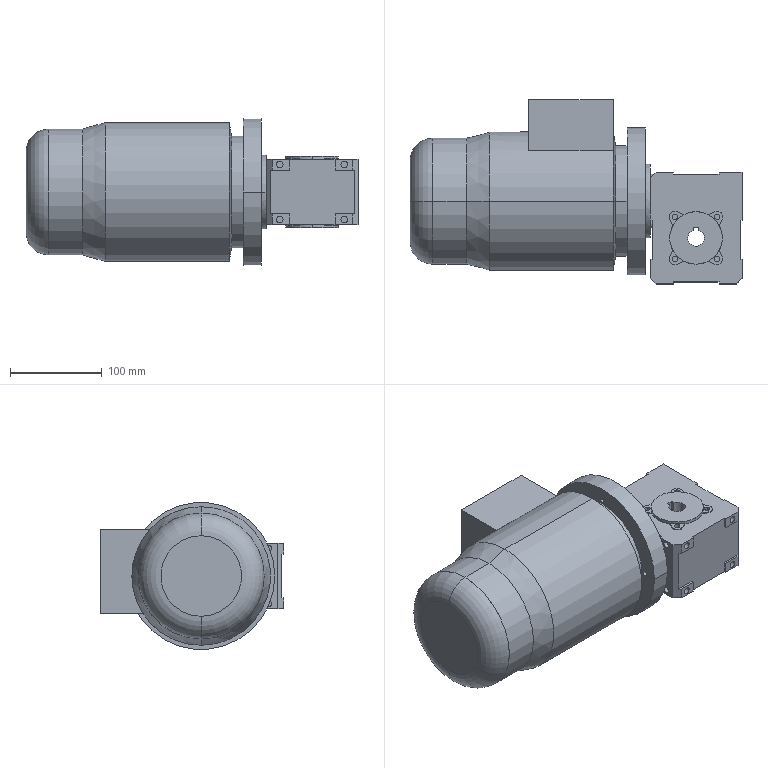Part | STEP file | Microwave Drying Flat Conveyor-worm gear reducer_mu40-base-10-b3 | 1 solid | 220 faces | box 361 x 200 x 160 mm | volume 5383182 mm3 | plane 119 | cylinder 95 | cone 4 | torus 2 | commonest cylinder face diameters 7 x28 6 x16 12.041 x12 5 x8 9.892 x5 8.473 x4